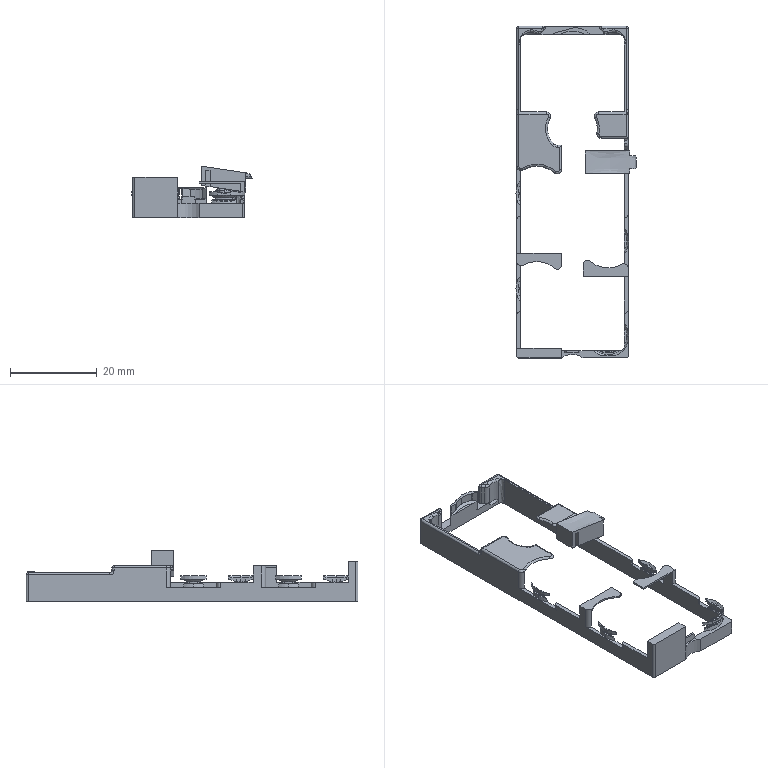Part | STEP file | I/O distribution box 23N4S1 | 2 solids | 273 faces | box 27.753 x 76.75 x 11.974 mm | volume 1445 mm3 | plane 110 | cylinder 85 | spline 42 | cone 34 | torus 2 | commonest cylinder face diameters 1 x26 2 x14 7.8 x7 8 x7 8.3 x7 9.6 x7